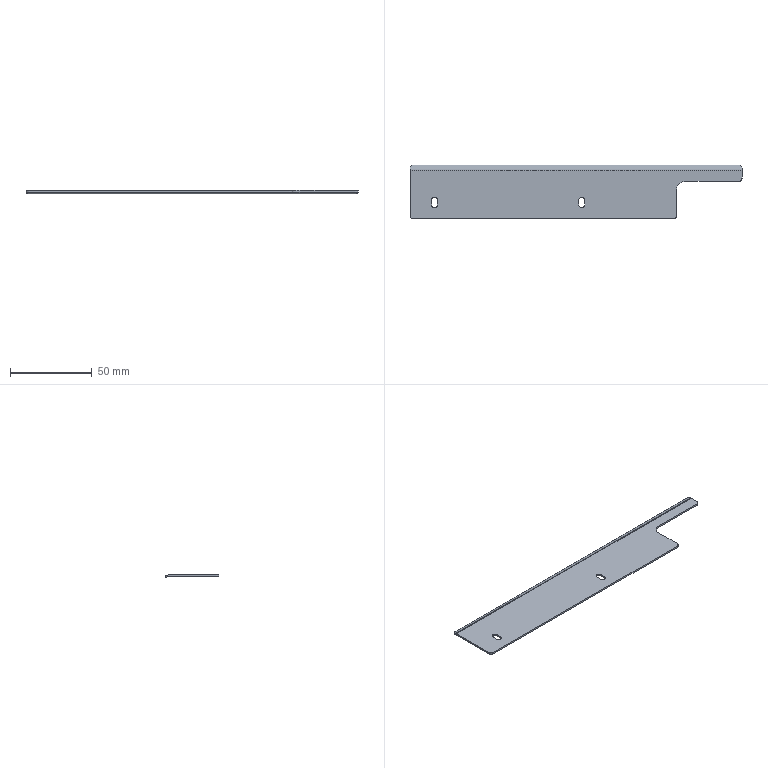Part | STEP file | 01-16 side baffle (Default) | 1 solid | 30 faces | box 203 x 32.995 x 1.966 mm | volume 5739 mm3 | plane 18 | cylinder 12 | commonest cylinder face diameters 4 x5 3.5 x4 1.473 x1 3.473 x1 10 x1
STEP:
#1=CARTESIAN_POINT('',(101.5,10.,0.));
#2=VERTEX_POINT('',#1);
#3=CARTESIAN_POINT('',(101.5,14.87,0.));
#4=VERTEX_POINT('',#3);
#5=CARTESIAN_POINT('',(101.5,15.,0.));
#6=DIRECTION('',(0.,1.,0.));
#7=VECTOR('',#6,1000.);
#8=LINE('',#5,#7);
#9=EDGE_CURVE('',#2,#4,#8,.T.);
#10=ORIENTED_EDGE('',*,*,#9,.F.);
#11=CARTESIAN_POINT('',(101.5,10.,-1.));
#12=VERTEX_POINT('',#11);
#13=CARTESIAN_POINT('',(101.5,10.,-1.));
#14=DIRECTION('',(0.,0.,-1.));
#15=VECTOR('',#14,1000.);
#16=LINE('',#13,#15);
#17=EDGE_CURVE('',#2,#12,#16,.T.);
#18=ORIENTED_EDGE('',*,*,#17,.T.);
#19=CARTESIAN_POINT('',(101.5,14.87,-1.));
#20=VERTEX_POINT('',#19);
#21=CARTESIAN_POINT('',(101.5,15.,-1.));
#22=DIRECTION('',(0.,1.,0.));
#23=VECTOR('',#22,1000.);
#24=LINE('',#21,#23);
#25=EDGE_CURVE('',#12,#20,#24,.T.);
#26=ORIENTED_EDGE('',*,*,#25,.T.);
#27=CARTESIAN_POINT('',(101.5,14.87,-1.));
#28=DIRECTION('',(0.,0.,1.));
#29=VECTOR('',#28,1000.);
#30=LINE('',#27,#29);
#31=EDGE_CURVE('',#20,#4,#30,.T.);
#32=ORIENTED_EDGE('',*,*,#31,.T.);
#33=EDGE_LOOP('',(#10,#18,#26,#32));
#34=FACE_OUTER_BOUND('',#33,.T.);
#35=CARTESIAN_POINT('',(101.5,15.,-1.));
#36=DIRECTION('',(1.,0.,0.));
#37=DIRECTION('',(0.,1.,0.));
#38=AXIS2_PLACEMENT_3D('',#35,#36,#37);
#39=PLANE('',#38);
#40=ADVANCED_FACE('',(#34),#39,.T.);
#41=CARTESIAN_POINT('',(5.25,-3.5,-1.));
#42=VERTEX_POINT('',#41);
#43=CARTESIAN_POINT('',(5.25,-6.5,-1.));
#44=VERTEX_POINT('',#43);
#45=CARTESIAN_POINT('',(5.25,-3.5,-1.));
#46=DIRECTION('',(0.,-1.,0.));
#47=VECTOR('',#46,1000.);
#48=LINE('',#45,#47);
#49=EDGE_CURVE('',#42,#44,#48,.T.);
#50=ORIENTED_EDGE('',*,*,#49,.F.);
#51=CARTESIAN_POINT('',(1.75,-3.5,-1.));
#52=VERTEX_POINT('',#51);
#53=CARTESIAN_POINT('',(3.5,-3.5,-1.));
#54=DIRECTION('',(0.,0.,-1.));
#55=DIRECTION('',(-1.,0.,0.));
#56=AXIS2_PLACEMENT_3D('',#53,#54,#55);
#57=CIRCLE('',#56,1.75);
#58=EDGE_CURVE('',#52,#42,#57,.T.);
#59=ORIENTED_EDGE('',*,*,#58,.F.);
#60=CARTESIAN_POINT('',(1.75,-6.5,-1.));
#61=VERTEX_POINT('',#60);
#62=CARTESIAN_POINT('',(1.75,-3.5,-1.));
#63=DIRECTION('',(0.,1.,0.));
#64=VECTOR('',#63,1000.);
#65=LINE('',#62,#64);
#66=EDGE_CURVE('',#61,#52,#65,.T.);
#67=ORIENTED_EDGE('',*,*,#66,.F.);
#68=CARTESIAN_POINT('',(3.5,-6.5,-1.));
#69=DIRECTION('',(0.,0.,-1.));
#70=DIRECTION('',(-1.,0.,0.));
#71=AXIS2_PLACEMENT_3D('',#68,#69,#70);
#72=CIRCLE('',#71,1.75);
#73=EDGE_CURVE('',#44,#61,#72,.T.);
#74=ORIENTED_EDGE('',*,*,#73,.F.);
#75=EDGE_LOOP('',(#50,#59,#67,#74));
#76=FACE_BOUND('',#75,.T.);
#77=CARTESIAN_POINT('',(-84.75,-3.5,-1.));
#78=VERTEX_POINT('',#77);
#79=CARTESIAN_POINT('',(-84.75,-6.5,-1.));
#80=VERTEX_POINT('',#79);
#81=CARTESIAN_POINT('',(-84.75,-3.5,-1.));
#82=DIRECTION('',(0.,-1.,0.));
#83=VECTOR('',#82,1000.);
#84=LINE('',#81,#83);
#85=EDGE_CURVE('',#78,#80,#84,.T.);
#86=ORIENTED_EDGE('',*,*,#85,.F.);
#87=CARTESIAN_POINT('',(-88.25,-3.5,-1.));
#88=VERTEX_POINT('',#87);
#89=CARTESIAN_POINT('',(-86.5,-3.5,-1.));
#90=DIRECTION('',(0.,0.,-1.));
#91=DIRECTION('',(-1.,0.,0.));
#92=AXIS2_PLACEMENT_3D('',#89,#90,#91);
#93=CIRCLE('',#92,1.75);
#94=EDGE_CURVE('',#88,#78,#93,.T.);
#95=ORIENTED_EDGE('',*,*,#94,.F.);
#96=CARTESIAN_POINT('',(-88.25,-6.5,-1.));
#97=VERTEX_POINT('',#96);
#98=CARTESIAN_POINT('',(-88.25,-3.5,-1.));
#99=DIRECTION('',(0.,1.,0.));
#100=VECTOR('',#99,1000.);
#101=LINE('',#98,#100);
#102=EDGE_CURVE('',#97,#88,#101,.T.);
#103=ORIENTED_EDGE('',*,*,#102,.F.);
#104=CARTESIAN_POINT('',(-86.5,-6.5,-1.));
#105=DIRECTION('',(0.,0.,-1.));
#106=DIRECTION('',(-1.,0.,0.));
#107=AXIS2_PLACEMENT_3D('',#104,#105,#106);
#108=CIRCLE('',#107,1.75);
#109=EDGE_CURVE('',#80,#97,#108,.T.);
#110=ORIENTED_EDGE('',*,*,#109,.F.);
#111=EDGE_LOOP('',(#86,#95,#103,#110));
#112=FACE_BOUND('',#111,.T.);
#113=ORIENTED_EDGE('',*,*,#25,.F.);
#114=CARTESIAN_POINT('',(99.5,8.,-1.));
#115=VERTEX_POINT('',#114);
#116=CARTESIAN_POINT('',(99.5,10.,-1.));
#117=DIRECTION('',(0.,0.,-1.));
#118=DIRECTION('',(1.,0.,0.));
#119=AXIS2_PLACEMENT_3D('',#116,#117,#118);
#120=CIRCLE('',#119,2.);
#121=EDGE_CURVE('',#12,#115,#120,.T.);
#122=ORIENTED_EDGE('',*,*,#121,.T.);
#123=CARTESIAN_POINT('',(66.5,8.,-1.));
#124=VERTEX_POINT('',#123);
#125=CARTESIAN_POINT('',(101.5,8.,-1.));
#126=DIRECTION('',(1.,0.,0.));
#127=VECTOR('',#126,1000.);
#128=LINE('',#125,#127);
#129=EDGE_CURVE('',#124,#115,#128,.T.);
#130=ORIENTED_EDGE('',*,*,#129,.F.);
#131=CARTESIAN_POINT('',(61.5,3.,-1.));
#132=VERTEX_POINT('',#131);
#133=CARTESIAN_POINT('',(66.5,3.,-1.));
#134=DIRECTION('',(0.,0.,-1.));
#135=DIRECTION('',(1.,0.,0.));
#136=AXIS2_PLACEMENT_3D('',#133,#134,#135);
#137=CIRCLE('',#136,5.);
#138=EDGE_CURVE('',#132,#124,#137,.T.);
#139=ORIENTED_EDGE('',*,*,#138,.F.);
#140=CARTESIAN_POINT('',(61.5,-13.,-1.));
#141=VERTEX_POINT('',#140);
#142=CARTESIAN_POINT('',(61.5,3.,-1.));
#143=DIRECTION('',(0.,1.,0.));
#144=VECTOR('',#143,1000.);
#145=LINE('',#142,#144);
#146=EDGE_CURVE('',#141,#132,#145,.T.);
#147=ORIENTED_EDGE('',*,*,#146,.F.);
#148=CARTESIAN_POINT('',(59.5,-15.,-1.));
#149=VERTEX_POINT('',#148);
#150=CARTESIAN_POINT('',(59.5,-13.,-1.));
#151=DIRECTION('',(0.,0.,-1.));
#152=DIRECTION('',(1.,0.,0.));
#153=AXIS2_PLACEMENT_3D('',#150,#151,#152);
#154=CIRCLE('',#153,2.);
#155=EDGE_CURVE('',#141,#149,#154,.T.);
#156=ORIENTED_EDGE('',*,*,#155,.T.);
#157=CARTESIAN_POINT('',(-99.5,-15.,-1.));
#158=VERTEX_POINT('',#157);
#159=CARTESIAN_POINT('',(-101.5,-15.,-1.));
#160=DIRECTION('',(1.,0.,0.));
#161=VECTOR('',#160,1000.);
#162=LINE('',#159,#161);
#163=EDGE_CURVE('',#158,#149,#162,.T.);
#164=ORIENTED_EDGE('',*,*,#163,.F.);
#165=CARTESIAN_POINT('',(-101.5,-13.,-1.));
#166=VERTEX_POINT('',#165);
#167=CARTESIAN_POINT('',(-99.5,-13.,-1.));
#168=DIRECTION('',(0.,0.,-1.));
#169=DIRECTION('',(1.,0.,0.));
#170=AXIS2_PLACEMENT_3D('',#167,#168,#169);
#171=CIRCLE('',#170,2.);
#172=EDGE_CURVE('',#158,#166,#171,.T.);
#173=ORIENTED_EDGE('',*,*,#172,.T.);
#174=CARTESIAN_POINT('',(-101.5,14.87,-1.));
#175=VERTEX_POINT('',#174);
#176=CARTESIAN_POINT('',(-101.5,15.,-1.));
#177=DIRECTION('',(0.,-1.,0.));
#178=VECTOR('',#177,1000.);
#179=LINE('',#176,#178);
#180=EDGE_CURVE('',#175,#166,#179,.T.);
#181=ORIENTED_EDGE('',*,*,#180,.F.);
#182=CARTESIAN_POINT('',(101.5,14.87,-1.));
#183=DIRECTION('',(-1.,0.,0.));
#184=VECTOR('',#183,1000.);
#185=LINE('',#182,#184);
#186=EDGE_CURVE('',#20,#175,#185,.T.);
#187=ORIENTED_EDGE('',*,*,#186,.F.);
#188=EDGE_LOOP('',(#113,#122,#130,#139,#147,#156,#164,#173,#181,#187));
#189=FACE_OUTER_BOUND('',#188,.T.);
#190=CARTESIAN_POINT('',(101.5,-15.,-1.));
#191=DIRECTION('',(0.,0.,1.));
#192=DIRECTION('',(1.,0.,0.));
#193=AXIS2_PLACEMENT_3D('',#190,#191,#192);
#194=PLANE('',#193);
#195=ADVANCED_FACE('',(#76,#112,#189),#194,.F.);
#196=CARTESIAN_POINT('',(5.25,-3.5,0.));
#197=VERTEX_POINT('',#196);
#198=CARTESIAN_POINT('',(1.75,-3.5,0.));
#199=VERTEX_POINT('',#198);
#200=CARTESIAN_POINT('',(3.5,-3.5,0.));
#201=DIRECTION('',(0.,0.,1.));
#202=DIRECTION('',(1.,0.,0.));
#203=AXIS2_PLACEMENT_3D('',#200,#201,#202);
#204=CIRCLE('',#203,1.75);
#205=EDGE_CURVE('',#197,#199,#204,.T.);
#206=ORIENTED_EDGE('',*,*,#205,.F.);
#207=CARTESIAN_POINT('',(5.25,-6.5,0.));
#208=VERTEX_POINT('',#207);
#209=CARTESIAN_POINT('',(5.25,-15.,0.));
#210=DIRECTION('',(0.,1.,0.));
#211=VECTOR('',#210,1000.);
#212=LINE('',#209,#211);
#213=EDGE_CURVE('',#208,#197,#212,.T.);
#214=ORIENTED_EDGE('',*,*,#213,.F.);
#215=CARTESIAN_POINT('',(1.75,-6.5,0.));
#216=VERTEX_POINT('',#215);
#217=CARTESIAN_POINT('',(3.5,-6.5,0.));
#218=DIRECTION('',(0.,0.,1.));
#219=DIRECTION('',(1.,0.,0.));
#220=AXIS2_PLACEMENT_3D('',#217,#218,#219);
#221=CIRCLE('',#220,1.75);
#222=EDGE_CURVE('',#216,#208,#221,.T.);
#223=ORIENTED_EDGE('',*,*,#222,.F.);
#224=CARTESIAN_POINT('',(1.75,-15.,0.));
#225=DIRECTION('',(0.,-1.,0.));
#226=VECTOR('',#225,1000.);
#227=LINE('',#224,#226);
#228=EDGE_CURVE('',#199,#216,#227,.T.);
#229=ORIENTED_EDGE('',*,*,#228,.F.);
#230=EDGE_LOOP('',(#206,#214,#223,#229));
#231=FACE_BOUND('',#230,.T.);
#232=CARTESIAN_POINT('',(-84.75,-3.5,0.));
#233=VERTEX_POINT('',#232);
#234=CARTESIAN_POINT('',(-88.25,-3.5,0.));
#235=VERTEX_POINT('',#234);
#236=CARTESIAN_POINT('',(-86.5,-3.5,0.));
#237=DIRECTION('',(0.,0.,1.));
#238=DIRECTION('',(1.,0.,0.));
#239=AXIS2_PLACEMENT_3D('',#236,#237,#238);
#240=CIRCLE('',#239,1.75);
#241=EDGE_CURVE('',#233,#235,#240,.T.);
#242=ORIENTED_EDGE('',*,*,#241,.F.);
#243=CARTESIAN_POINT('',(-84.75,-6.5,0.));
#244=VERTEX_POINT('',#243);
#245=CARTESIAN_POINT('',(-84.75,-15.,0.));
#246=DIRECTION('',(0.,1.,0.));
#247=VECTOR('',#246,1000.);
#248=LINE('',#245,#247);
#249=EDGE_CURVE('',#244,#233,#248,.T.);
#250=ORIENTED_EDGE('',*,*,#249,.F.);
#251=CARTESIAN_POINT('',(-88.25,-6.5,0.));
#252=VERTEX_POINT('',#251);
#253=CARTESIAN_POINT('',(-86.5,-6.5,0.));
#254=DIRECTION('',(0.,0.,1.));
#255=DIRECTION('',(1.,0.,0.));
#256=AXIS2_PLACEMENT_3D('',#253,#254,#255);
#257=CIRCLE('',#256,1.75);
#258=EDGE_CURVE('',#252,#244,#257,.T.);
#259=ORIENTED_EDGE('',*,*,#258,.F.);
#260=CARTESIAN_POINT('',(-88.25,-15.,0.));
#261=DIRECTION('',(0.,-1.,0.));
#262=VECTOR('',#261,1000.);
#263=LINE('',#260,#262);
#264=EDGE_CURVE('',#235,#252,#263,.T.);
#265=ORIENTED_EDGE('',*,*,#264,.F.);
#266=EDGE_LOOP('',(#242,#250,#259,#265));
#267=FACE_BOUND('',#266,.T.);
#268=CARTESIAN_POINT('',(99.5,8.,0.));
#269=VERTEX_POINT('',#268);
#270=CARTESIAN_POINT('',(66.5,8.,0.));
#271=VERTEX_POINT('',#270);
#272=CARTESIAN_POINT('',(101.5,8.,0.));
#273=DIRECTION('',(-1.,0.,0.));
#274=VECTOR('',#273,1000.);
#275=LINE('',#272,#274);
#276=EDGE_CURVE('',#269,#271,#275,.T.);
#277=ORIENTED_EDGE('',*,*,#276,.F.);
#278=CARTESIAN_POINT('',(99.5,10.,0.));
#279=DIRECTION('',(0.,0.,1.));
#280=DIRECTION('',(1.,0.,0.));
#281=AXIS2_PLACEMENT_3D('',#278,#279,#280);
#282=CIRCLE('',#281,2.);
#283=EDGE_CURVE('',#269,#2,#282,.T.);
#284=ORIENTED_EDGE('',*,*,#283,.T.);
#285=ORIENTED_EDGE('',*,*,#9,.T.);
#286=CARTESIAN_POINT('',(-101.5,14.87,0.));
#287=VERTEX_POINT('',#286);
#288=CARTESIAN_POINT('',(101.5,14.87,0.));
#289=DIRECTION('',(-1.,0.,0.));
#290=VECTOR('',#289,1000.);
#291=LINE('',#288,#290);
#292=EDGE_CURVE('',#4,#287,#291,.T.);
#293=ORIENTED_EDGE('',*,*,#292,.T.);
#294=CARTESIAN_POINT('',(-101.5,-13.,0.));
#295=VERTEX_POINT('',#294);
#296=CARTESIAN_POINT('',(-101.5,15.,0.));
#297=DIRECTION('',(0.,-1.,0.));
#298=VECTOR('',#297,1000.);
#299=LINE('',#296,#298);
#300=EDGE_CURVE('',#287,#295,#299,.T.);
#301=ORIENTED_EDGE('',*,*,#300,.T.);
#302=CARTESIAN_POINT('',(-99.5,-15.,0.));
#303=VERTEX_POINT('',#302);
#304=CARTESIAN_POINT('',(-99.5,-13.,0.));
#305=DIRECTION('',(0.,0.,1.));
#306=DIRECTION('',(1.,0.,0.));
#307=AXIS2_PLACEMENT_3D('',#304,#305,#306);
#308=CIRCLE('',#307,2.);
#309=EDGE_CURVE('',#295,#303,#308,.T.);
#310=ORIENTED_EDGE('',*,*,#309,.T.);
#311=CARTESIAN_POINT('',(59.5,-15.,0.));
#312=VERTEX_POINT('',#311);
#313=CARTESIAN_POINT('',(-101.5,-15.,0.));
#314=DIRECTION('',(1.,0.,0.));
#315=VECTOR('',#314,1000.);
#316=LINE('',#313,#315);
#317=EDGE_CURVE('',#303,#312,#316,.T.);
#318=ORIENTED_EDGE('',*,*,#317,.T.);
#319=CARTESIAN_POINT('',(61.5,-13.,0.));
#320=VERTEX_POINT('',#319);
#321=CARTESIAN_POINT('',(59.5,-13.,0.));
#322=DIRECTION('',(0.,0.,1.));
#323=DIRECTION('',(1.,0.,0.));
#324=AXIS2_PLACEMENT_3D('',#321,#322,#323);
#325=CIRCLE('',#324,2.);
#326=EDGE_CURVE('',#312,#320,#325,.T.);
#327=ORIENTED_EDGE('',*,*,#326,.T.);
#328=CARTESIAN_POINT('',(61.5,3.,0.));
#329=VERTEX_POINT('',#328);
#330=CARTESIAN_POINT('',(61.5,-15.,0.));
#331=DIRECTION('',(0.,-1.,0.));
#332=VECTOR('',#331,1000.);
#333=LINE('',#330,#332);
#334=EDGE_CURVE('',#329,#320,#333,.T.);
#335=ORIENTED_EDGE('',*,*,#334,.F.);
#336=CARTESIAN_POINT('',(66.5,3.,0.));
#337=DIRECTION('',(0.,0.,1.));
#338=DIRECTION('',(1.,0.,0.));
#339=AXIS2_PLACEMENT_3D('',#336,#337,#338);
#340=CIRCLE('',#339,5.);
#341=EDGE_CURVE('',#271,#329,#340,.T.);
#342=ORIENTED_EDGE('',*,*,#341,.F.);
#343=EDGE_LOOP('',(#277,#284,#285,#293,#301,#310,#318,#327,#335,#342));
#344=FACE_OUTER_BOUND('',#343,.T.);
#345=CARTESIAN_POINT('',(101.5,-15.,0.));
#346=DIRECTION('',(0.,0.,1.));
#347=DIRECTION('',(1.,0.,0.));
#348=AXIS2_PLACEMENT_3D('',#345,#346,#347);
#349=PLANE('',#348);
#350=ADVANCED_FACE('',(#231,#267,#344),#349,.T.);
#351=ORIENTED_EDGE('',*,*,#163,.T.);
#352=CARTESIAN_POINT('',(59.5,-15.,0.));
#353=DIRECTION('',(0.,0.,1.));
#354=VECTOR('',#353,1000.);
#355=LINE('',#352,#354);
#356=EDGE_CURVE('',#149,#312,#355,.T.);
#357=ORIENTED_EDGE('',*,*,#356,.T.);
#358=ORIENTED_EDGE('',*,*,#317,.F.);
#359=CARTESIAN_POINT('',(-99.5,-15.,-1.));
#360=DIRECTION('',(0.,0.,-1.));
#361=VECTOR('',#360,1000.);
#362=LINE('',#359,#361);
#363=EDGE_CURVE('',#303,#158,#362,.T.);
#364=ORIENTED_EDGE('',*,*,#363,.T.);
#365=EDGE_LOOP('',(#351,#357,#358,#364));
#366=FACE_OUTER_BOUND('',#365,.T.);
#367=CARTESIAN_POINT('',(-101.5,-15.,-1.));
#368=DIRECTION('',(0.,-1.,0.));
#369=DIRECTION('',(0.,0.,-1.));
#370=AXIS2_PLACEMENT_3D('',#367,#368,#369);
#371=PLANE('',#370);
#372=ADVANCED_FACE('',(#366),#371,.T.);
#373=ORIENTED_EDGE('',*,*,#180,.T.);
#374=CARTESIAN_POINT('',(-101.5,-13.,-1.));
#375=DIRECTION('',(0.,0.,1.));
#376=VECTOR('',#375,1000.);
#377=LINE('',#374,#376);
#378=EDGE_CURVE('',#166,#295,#377,.T.);
#379=ORIENTED_EDGE('',*,*,#378,.T.);
#380=ORIENTED_EDGE('',*,*,#300,.F.);
#381=CARTESIAN_POINT('',(-101.5,14.87,-1.));
#382=DIRECTION('',(0.,0.,1.));
#383=VECTOR('',#382,1000.);
#384=LINE('',#381,#383);
#385=EDGE_CURVE('',#175,#287,#384,.T.);
#386=ORIENTED_EDGE('',*,*,#385,.F.);
#387=EDGE_LOOP('',(#373,#379,#380,#386));
#388=FACE_OUTER_BOUND('',#387,.T.);
#389=CARTESIAN_POINT('',(-101.5,15.,-1.));
#390=DIRECTION('',(-1.,0.,0.));
#391=DIRECTION('',(0.,0.,1.));
#392=AXIS2_PLACEMENT_3D('',#389,#390,#391);
#393=PLANE('',#392);
#394=ADVANCED_FACE('',(#388),#393,.T.);
#395=CARTESIAN_POINT('',(-101.5,15.122,-1.044));
#396=VERTEX_POINT('',#395);
#397=CARTESIAN_POINT('',(-101.5,15.464,-0.1047));
#398=VERTEX_POINT('',#397);
#399=CARTESIAN_POINT('',(-101.5,15.122,-1.044));
#400=DIRECTION('',(0.,0.342,0.9397));
#401=VECTOR('',#400,1000.);
#402=LINE('',#399,#401);
#403=EDGE_CURVE('',#396,#398,#402,.T.);
#404=ORIENTED_EDGE('',*,*,#403,.F.);
#405=CARTESIAN_POINT('',(-101.5,14.87,-1.737));
#406=DIRECTION('',(-1.,0.,0.));
#407=DIRECTION('',(0.,0.,-1.));
#408=AXIS2_PLACEMENT_3D('',#405,#406,#407);
#409=CIRCLE('',#408,0.7366);
#410=EDGE_CURVE('',#175,#396,#409,.T.);
#411=ORIENTED_EDGE('',*,*,#410,.F.);
#412=ORIENTED_EDGE('',*,*,#385,.T.);
#413=CARTESIAN_POINT('',(-101.5,14.87,-1.737));
#414=DIRECTION('',(-1.,0.,0.));
#415=DIRECTION('',(0.,0.,-1.));
#416=AXIS2_PLACEMENT_3D('',#413,#414,#415);
#417=CIRCLE('',#416,1.737);
#418=EDGE_CURVE('',#287,#398,#417,.T.);
#419=ORIENTED_EDGE('',*,*,#418,.T.);
#420=EDGE_LOOP('',(#404,#411,#412,#419));
#421=FACE_OUTER_BOUND('',#420,.T.);
#422=CARTESIAN_POINT('',(-101.5,14.87,-1.737));
#423=DIRECTION('',(-1.,0.,0.));
#424=DIRECTION('',(0.,0.,1.));
#425=AXIS2_PLACEMENT_3D('',#422,#423,#424);
#426=PLANE('',#425);
#427=ADVANCED_FACE('',(#421),#426,.T.);
#428=CARTESIAN_POINT('',(101.5,15.122,-1.044));
#429=VERTEX_POINT('',#428);
#430=CARTESIAN_POINT('',(101.5,14.87,-1.737));
#431=DIRECTION('',(1.,0.,0.));
#432=DIRECTION('',(0.,0.,-1.));
#433=AXIS2_PLACEMENT_3D('',#430,#431,#432);
#434=CIRCLE('',#433,0.7366);
#435=EDGE_CURVE('',#429,#20,#434,.T.);
#436=ORIENTED_EDGE('',*,*,#435,.F.);
#437=CARTESIAN_POINT('',(101.5,15.464,-0.1047));
#438=VERTEX_POINT('',#437);
#439=CARTESIAN_POINT('',(101.5,15.122,-1.044));
#440=DIRECTION('',(0.,0.342,0.9397));
#441=VECTOR('',#440,1000.);
#442=LINE('',#439,#441);
#443=EDGE_CURVE('',#429,#438,#442,.T.);
#444=ORIENTED_EDGE('',*,*,#443,.T.);
#445=CARTESIAN_POINT('',(101.5,14.87,-1.737));
#446=DIRECTION('',(1.,0.,0.));
#447=DIRECTION('',(0.,0.,-1.));
#448=AXIS2_PLACEMENT_3D('',#445,#446,#447);
#449=CIRCLE('',#448,1.737);
#450=EDGE_CURVE('',#438,#4,#449,.T.);
#451=ORIENTED_EDGE('',*,*,#450,.T.);
#452=ORIENTED_EDGE('',*,*,#31,.F.);
#453=EDGE_LOOP('',(#436,#444,#451,#452));
#454=FACE_OUTER_BOUND('',#453,.T.);
#455=CARTESIAN_POINT('',(101.5,14.87,-1.737));
#456=DIRECTION('',(-1.,0.,0.));
#457=DIRECTION('',(0.,0.,1.));
#458=AXIS2_PLACEMENT_3D('',#455,#456,#457);
#459=PLANE('',#458);
#460=ADVANCED_FACE('',(#454),#459,.F.);
#461=ORIENTED_EDGE('',*,*,#292,.F.);
#462=ORIENTED_EDGE('',*,*,#450,.F.);
#463=CARTESIAN_POINT('',(101.5,15.464,-0.1047));
#464=DIRECTION('',(-1.,0.,0.));
#465=VECTOR('',#464,1000.);
#466=LINE('',#463,#465);
#467=EDGE_CURVE('',#438,#398,#466,.T.);
#468=ORIENTED_EDGE('',*,*,#467,.T.);
#469=ORIENTED_EDGE('',*,*,#418,.F.);
#470=EDGE_LOOP('',(#461,#462,#468,#469));
#471=FACE_OUTER_BOUND('',#470,.T.);
#472=CARTESIAN_POINT('',(101.5,14.87,-1.737));
#473=DIRECTION('',(1.,0.,0.));
#474=DIRECTION('',(0.,0.342,0.9397));
#475=AXIS2_PLACEMENT_3D('',#472,#473,#474);
#476=CYLINDRICAL_SURFACE('',#475,1.737);
#477=ADVANCED_FACE('',(#471),#476,.T.);
#478=ORIENTED_EDGE('',*,*,#186,.T.);
#479=ORIENTED_EDGE('',*,*,#410,.T.);
#480=CARTESIAN_POINT('',(-101.5,15.122,-1.044));
#481=DIRECTION('',(1.,0.,0.));
#482=VECTOR('',#481,1000.);
#483=LINE('',#480,#482);
#484=EDGE_CURVE('',#396,#429,#483,.T.);
#485=ORIENTED_EDGE('',*,*,#484,.T.);
#486=ORIENTED_EDGE('',*,*,#435,.T.);
#487=EDGE_LOOP('',(#478,#479,#485,#486));
#488=FACE_OUTER_BOUND('',#487,.T.);
#489=CARTESIAN_POINT('',(101.5,14.87,-1.737));
#490=DIRECTION('',(1.,0.,0.));
#491=DIRECTION('',(0.,0.342,0.9397));
#492=AXIS2_PLACEMENT_3D('',#489,#490,#491);
#493=CYLINDRICAL_SURFACE('',#492,0.7366);
#494=ADVANCED_FACE('',(#488),#493,.F.);
#495=CARTESIAN_POINT('',(101.5,15.774,-1.282));
#496=VERTEX_POINT('',#495);
#497=CARTESIAN_POINT('',(101.5,17.653,-1.966));
#498=DIRECTION('',(0.,0.9397,-0.342));
#499=VECTOR('',#498,1000.);
#500=LINE('',#497,#499);
#501=EDGE_CURVE('',#429,#496,#500,.T.);
#502=ORIENTED_EDGE('',*,*,#501,.T.);
#503=CARTESIAN_POINT('',(101.5,16.116,-0.342));
#504=VERTEX_POINT('',#503);
#505=CARTESIAN_POINT('',(101.5,16.116,-0.342));
#506=DIRECTION('',(0.,0.342,0.9397));
#507=VECTOR('',#506,1000.);
#508=LINE('',#505,#507);
#509=EDGE_CURVE('',#496,#504,#508,.T.);
#510=ORIENTED_EDGE('',*,*,#509,.T.);
#511=CARTESIAN_POINT('',(101.5,17.995,-1.026));
#512=DIRECTION('',(0.,0.9397,-0.342));
#513=VECTOR('',#512,1000.);
#514=LINE('',#511,#513);
#515=EDGE_CURVE('',#438,#504,#514,.T.);
#516=ORIENTED_EDGE('',*,*,#515,.F.);
#517=ORIENTED_EDGE('',*,*,#443,.F.);
#518=EDGE_LOOP('',(#502,#510,#516,#517));
#519=FACE_OUTER_BOUND('',#518,.T.);
#520=CARTESIAN_POINT('',(101.5,17.995,-1.026));
#521=DIRECTION('',(-1.,0.,0.));
#522=DIRECTION('',(0.,0.,1.));
#523=AXIS2_PLACEMENT_3D('',#520,#521,#522);
#524=PLANE('',#523);
#525=ADVANCED_FACE('',(#519),#524,.F.);
#526=CARTESIAN_POINT('',(-101.5,16.116,-0.342));
#527=VERTEX_POINT('',#526);
#528=CARTESIAN_POINT('',(-101.5,15.342,-0.06031));
#529=DIRECTION('',(0.,-0.9397,0.342));
#530=VECTOR('',#529,1000.);
#531=LINE('',#528,#530);
#532=EDGE_CURVE('',#527,#398,#531,.T.);
#533=ORIENTED_EDGE('',*,*,#532,.F.);
#534=CARTESIAN_POINT('',(-101.5,15.774,-1.282));
#535=VERTEX_POINT('',#534);
#536=CARTESIAN_POINT('',(-101.5,16.116,-0.342));
#537=DIRECTION('',(0.,-0.342,-0.9397));
#538=VECTOR('',#537,1000.);
#539=LINE('',#536,#538);
#540=EDGE_CURVE('',#527,#535,#539,.T.);
#541=ORIENTED_EDGE('',*,*,#540,.T.);
#542=CARTESIAN_POINT('',(-101.5,15.,-1.));
#543=DIRECTION('',(0.,-0.9397,0.342));
#544=VECTOR('',#543,1000.);
#545=LINE('',#542,#544);
#546=EDGE_CURVE('',#535,#396,#545,.T.);
#547=ORIENTED_EDGE('',*,*,#546,.T.);
#548=ORIENTED_EDGE('',*,*,#403,.T.);
#549=EDGE_LOOP('',(#533,#541,#547,#548));
#550=FACE_OUTER_BOUND('',#549,.T.);
#551=CARTESIAN_POINT('',(-101.5,15.342,-0.06031));
#552=DIRECTION('',(1.,0.,0.));
#553=DIRECTION('',(0.,0.,-1.));
#554=AXIS2_PLACEMENT_3D('',#551,#552,#553);
#555=PLANE('',#554);
#556=ADVANCED_FACE('',(#550),#555,.F.);
#557=ORIENTED_EDGE('',*,*,#515,.T.);
#558=CARTESIAN_POINT('',(99.5,17.995,-1.026));
#559=VERTEX_POINT('',#558);
#560=CARTESIAN_POINT('',(99.5,16.116,-0.342));
#561=DIRECTION('',(0.,0.342,0.9397));
#562=DIRECTION('',(0.,0.9397,-0.342));
#563=AXIS2_PLACEMENT_3D('',#560,#561,#562);
#564=CIRCLE('',#563,2.);
#565=EDGE_CURVE('',#504,#559,#564,.T.);
#566=ORIENTED_EDGE('',*,*,#565,.T.);
#567=CARTESIAN_POINT('',(-99.5,17.995,-1.026));
#568=VERTEX_POINT('',#567);
#569=CARTESIAN_POINT('',(-101.5,17.995,-1.026));
#570=DIRECTION('',(-1.,0.,0.));
#571=VECTOR('',#570,1000.);
#572=LINE('',#569,#571);
#573=EDGE_CURVE('',#559,#568,#572,.T.);
#574=ORIENTED_EDGE('',*,*,#573,.T.);
#575=CARTESIAN_POINT('',(-99.5,16.116,-0.342));
#576=DIRECTION('',(0.,0.342,0.9397));
#577=DIRECTION('',(0.,0.9397,-0.342));
#578=AXIS2_PLACEMENT_3D('',#575,#576,#577);
#579=CIRCLE('',#578,2.);
#580=EDGE_CURVE('',#568,#527,#579,.T.);
#581=ORIENTED_EDGE('',*,*,#580,.T.);
#582=ORIENTED_EDGE('',*,*,#532,.T.);
#583=ORIENTED_EDGE('',*,*,#467,.F.);
#584=EDGE_LOOP('',(#557,#566,#574,#581,#582,#583));
#585=FACE_OUTER_BOUND('',#584,.T.);
#586=CARTESIAN_POINT('',(101.5,15.342,-0.06031));
#587=DIRECTION('',(0.,-0.342,-0.9397));
#588=DIRECTION('',(0.,0.9397,-0.342));
#589=AXIS2_PLACEMENT_3D('',#586,#587,#588);
#590=PLANE('',#589);
#591=ADVANCED_FACE('',(#585),#590,.F.);
#592=CARTESIAN_POINT('',(99.5,17.653,-1.966));
#593=VERTEX_POINT('',#592);
#594=CARTESIAN_POINT('',(-99.5,17.653,-1.966));
#595=VERTEX_POINT('',#594);
#596=CARTESIAN_POINT('',(-101.5,17.653,-1.966));
#597=DIRECTION('',(-1.,0.,0.));
#598=VECTOR('',#597,1000.);
#599=LINE('',#596,#598);
#600=EDGE_CURVE('',#593,#595,#599,.T.);
#601=ORIENTED_EDGE('',*,*,#600,.F.);
#602=CARTESIAN_POINT('',(99.5,15.774,-1.282));
#603=DIRECTION('',(0.,-0.342,-0.9397));
#604=DIRECTION('',(0.,0.9397,-0.342));
#605=AXIS2_PLACEMENT_3D('',#602,#603,#604);
#606=CIRCLE('',#605,2.);
#607=EDGE_CURVE('',#593,#496,#606,.T.);
#608=ORIENTED_EDGE('',*,*,#607,.T.);
#609=ORIENTED_EDGE('',*,*,#501,.F.);
#610=ORIENTED_EDGE('',*,*,#484,.F.);
#611=ORIENTED_EDGE('',*,*,#546,.F.);
#612=CARTESIAN_POINT('',(-99.5,15.774,-1.282));
#613=DIRECTION('',(0.,-0.342,-0.9397));
#614=DIRECTION('',(0.,0.9397,-0.342));
#615=AXIS2_PLACEMENT_3D('',#612,#613,#614);
#616=CIRCLE('',#615,2.);
#617=EDGE_CURVE('',#535,#595,#616,.T.);
#618=ORIENTED_EDGE('',*,*,#617,.T.);
#619=EDGE_LOOP('',(#601,#608,#609,#610,#611,#618));
#620=FACE_OUTER_BOUND('',#619,.T.);
#621=CARTESIAN_POINT('',(101.5,15.,-1.));
#622=DIRECTION('',(0.,-0.342,-0.9397));
#623=DIRECTION('',(0.,0.9397,-0.342));
#624=AXIS2_PLACEMENT_3D('',#621,#622,#623);
#625=PLANE('',#624);
#626=ADVANCED_FACE('',(#620),#625,.T.);
#627=ORIENTED_EDGE('',*,*,#573,.F.);
#628=CARTESIAN_POINT('',(99.5,17.995,-1.026));
#629=DIRECTION('',(0.,-0.342,-0.9397));
#630=VECTOR('',#629,1000.);
#631=LINE('',#628,#630);
#632=EDGE_CURVE('',#559,#593,#631,.T.);
#633=ORIENTED_EDGE('',*,*,#632,.T.);
#634=ORIENTED_EDGE('',*,*,#600,.T.);
#635=CARTESIAN_POINT('',(-99.5,17.995,-1.026));
#636=DIRECTION('',(0.,0.342,0.9397));
#637=VECTOR('',#636,1000.);
#638=LINE('',#635,#637);
#639=EDGE_CURVE('',#595,#568,#638,.T.);
#640=ORIENTED_EDGE('',*,*,#639,.T.);
#641=EDGE_LOOP('',(#627,#633,#634,#640));
#642=FACE_OUTER_BOUND('',#641,.T.);
#643=CARTESIAN_POINT('',(-101.5,17.995,-1.026));
#644=DIRECTION('',(0.,-0.9397,0.342));
#645=DIRECTION('',(0.,-0.342,-0.9397));
#646=AXIS2_PLACEMENT_3D('',#643,#644,#645);
#647=PLANE('',#646);
#648=ADVANCED_FACE('',(#642),#647,.F.);
#649=ORIENTED_EDGE('',*,*,#172,.F.);
#650=ORIENTED_EDGE('',*,*,#363,.F.);
#651=ORIENTED_EDGE('',*,*,#309,.F.);
#652=ORIENTED_EDGE('',*,*,#378,.F.);
#653=EDGE_LOOP('',(#649,#650,#651,#652));
#654=FACE_OUTER_BOUND('',#653,.T.);
#655=CARTESIAN_POINT('',(-99.5,-13.,-1.));
#656=DIRECTION('',(0.,0.,1.));
#657=DIRECTION('',(1.,0.,0.));
#658=AXIS2_PLACEMENT_3D('',#655,#656,#657);
#659=CYLINDRICAL_SURFACE('',#658,2.);
#660=ADVANCED_FACE('',(#654),#659,.T.);
#661=ORIENTED_EDGE('',*,*,#565,.F.);
#662=ORIENTED_EDGE('',*,*,#509,.F.);
#663=ORIENTED_EDGE('',*,*,#607,.F.);
#664=ORIENTED_EDGE('',*,*,#632,.F.);
#665=EDGE_LOOP('',(#661,#662,#663,#664));
#666=FACE_OUTER_BOUND('',#665,.T.);
#667=CARTESIAN_POINT('',(99.5,16.116,-0.342));
#668=DIRECTION('',(0.,-0.342,-0.9397));
#669=DIRECTION('',(0.,0.9397,-0.342));
#670=AXIS2_PLACEMENT_3D('',#667,#668,#669);
#671=CYLINDRICAL_SURFACE('',#670,2.);
#672=ADVANCED_FACE('',(#666),#671,.T.);
#673=ORIENTED_EDGE('',*,*,#580,.F.);
#674=ORIENTED_EDGE('',*,*,#639,.F.);
#675=ORIENTED_EDGE('',*,*,#617,.F.);
#676=ORIENTED_EDGE('',*,*,#540,.F.);
#677=EDGE_LOOP('',(#673,#674,#675,#676));
#678=FACE_OUTER_BOUND('',#677,.T.);
#679=CARTESIAN_POINT('',(-99.5,16.116,-0.342));
#680=DIRECTION('',(0.,-0.342,-0.9397));
#681=DIRECTION('',(0.,0.9397,-0.342));
#682=AXIS2_PLACEMENT_3D('',#679,#680,#681);
#683=CYLINDRICAL_SURFACE('',#682,2.);
#684=ADVANCED_FACE('',(#678),#683,.T.);
#685=ORIENTED_EDGE('',*,*,#129,.T.);
#686=CARTESIAN_POINT('',(99.5,8.,0.));
#687=DIRECTION('',(0.,0.,1.));
#688=VECTOR('',#687,1000.);
#689=LINE('',#686,#688);
#690=EDGE_CURVE('',#115,#269,#689,.T.);
#691=ORIENTED_EDGE('',*,*,#690,.T.);
#692=ORIENTED_EDGE('',*,*,#276,.T.);
#693=CARTESIAN_POINT('',(66.5,8.,9.));
#694=DIRECTION('',(0.,0.,-1.));
#695=VECTOR('',#694,1000.);
#696=LINE('',#693,#695);
#697=EDGE_CURVE('',#271,#124,#696,.T.);
#698=ORIENTED_EDGE('',*,*,#697,.T.);
#699=EDGE_LOOP('',(#685,#691,#692,#698));
#700=FACE_OUTER_BOUND('',#699,.T.);
#701=CARTESIAN_POINT('',(101.5,8.,9.));
#702=DIRECTION('',(0.,1.,0.));
#703=DIRECTION('',(0.,0.,1.));
#704=AXIS2_PLACEMENT_3D('',#701,#702,#703);
#705=PLANE('',#704);
#706=ADVANCED_FACE('',(#700),#705,.F.);
#707=ORIENTED_EDGE('',*,*,#341,.T.);
#708=CARTESIAN_POINT('',(61.5,3.,9.));
#709=DIRECTION('',(0.,0.,-1.));
#710=VECTOR('',#709,1000.);
#711=LINE('',#708,#710);
#712=EDGE_CURVE('',#329,#132,#711,.T.);
#713=ORIENTED_EDGE('',*,*,#712,.T.);
#714=ORIENTED_EDGE('',*,*,#138,.T.);
#715=ORIENTED_EDGE('',*,*,#697,.F.);
#716=EDGE_LOOP('',(#707,#713,#714,#715));
#717=FACE_OUTER_BOUND('',#716,.T.);
#718=CARTESIAN_POINT('',(66.5,3.,9.));
#719=DIRECTION('',(0.,0.,-1.));
#720=DIRECTION('',(-1.,0.,0.));
#721=AXIS2_PLACEMENT_3D('',#718,#719,#720);
#722=CYLINDRICAL_SURFACE('',#721,5.);
#723=ADVANCED_FACE('',(#717),#722,.F.);
#724=ORIENTED_EDGE('',*,*,#334,.T.);
#725=CARTESIAN_POINT('',(61.5,-13.,-1.));
#726=DIRECTION('',(0.,0.,-1.));
#727=VECTOR('',#726,1000.);
#728=LINE('',#725,#727);
#729=EDGE_CURVE('',#320,#141,#728,.T.);
#730=ORIENTED_EDGE('',*,*,#729,.T.);
#731=ORIENTED_EDGE('',*,*,#146,.T.);
#732=ORIENTED_EDGE('',*,*,#712,.F.);
#733=EDGE_LOOP('',(#724,#730,#731,#732));
#734=FACE_OUTER_BOUND('',#733,.T.);
#735=CARTESIAN_POINT('',(61.5,3.,9.));
#736=DIRECTION('',(-1.,0.,0.));
#737=DIRECTION('',(0.,0.,1.));
#738=AXIS2_PLACEMENT_3D('',#735,#736,#737);
#739=PLANE('',#738);
#740=ADVANCED_FACE('',(#734),#739,.F.);
#741=ORIENTED_EDGE('',*,*,#241,.T.);
#742=CARTESIAN_POINT('',(-88.25,-3.5,9.));
#743=DIRECTION('',(0.,0.,-1.));
#744=VECTOR('',#743,1000.);
#745=LINE('',#742,#744);
#746=EDGE_CURVE('',#235,#88,#745,.T.);
#747=ORIENTED_EDGE('',*,*,#746,.T.);
#748=ORIENTED_EDGE('',*,*,#94,.T.);
#749=CARTESIAN_POINT('',(-84.75,-3.5,9.));
#750=DIRECTION('',(0.,0.,-1.));
#751=VECTOR('',#750,1000.);
#752=LINE('',#749,#751);
#753=EDGE_CURVE('',#233,#78,#752,.T.);
#754=ORIENTED_EDGE('',*,*,#753,.F.);
#755=EDGE_LOOP('',(#741,#747,#748,#754));
#756=FACE_OUTER_BOUND('',#755,.T.);
#757=CARTESIAN_POINT('',(-86.5,-3.5,9.));
#758=DIRECTION('',(0.,0.,-1.));
#759=DIRECTION('',(-1.,0.,0.));
#760=AXIS2_PLACEMENT_3D('',#757,#758,#759);
#761=CYLINDRICAL_SURFACE('',#760,1.75);
#762=ADVANCED_FACE('',(#756),#761,.F.);
#763=ORIENTED_EDGE('',*,*,#264,.T.);
#764=CARTESIAN_POINT('',(-88.25,-6.5,9.));
#765=DIRECTION('',(0.,0.,-1.));
#766=VECTOR('',#765,1000.);
#767=LINE('',#764,#766);
#768=EDGE_CURVE('',#252,#97,#767,.T.);
#769=ORIENTED_EDGE('',*,*,#768,.T.);
#770=ORIENTED_EDGE('',*,*,#102,.T.);
#771=ORIENTED_EDGE('',*,*,#746,.F.);
#772=EDGE_LOOP('',(#763,#769,#770,#771));
#773=FACE_OUTER_BOUND('',#772,.T.);
#774=CARTESIAN_POINT('',(-88.25,-3.5,9.));
#775=DIRECTION('',(-1.,0.,0.));
#776=DIRECTION('',(0.,0.,1.));
#777=AXIS2_PLACEMENT_3D('',#774,#775,#776);
#778=PLANE('',#777);
#779=ADVANCED_FACE('',(#773),#778,.F.);
#780=ORIENTED_EDGE('',*,*,#258,.T.);
#781=CARTESIAN_POINT('',(-84.75,-6.5,9.));
#782=DIRECTION('',(0.,0.,-1.));
#783=VECTOR('',#782,1000.);
#784=LINE('',#781,#783);
#785=EDGE_CURVE('',#244,#80,#784,.T.);
#786=ORIENTED_EDGE('',*,*,#785,.T.);
#787=ORIENTED_EDGE('',*,*,#109,.T.);
#788=ORIENTED_EDGE('',*,*,#768,.F.);
#789=EDGE_LOOP('',(#780,#786,#787,#788));
#790=FACE_OUTER_BOUND('',#789,.T.);
#791=CARTESIAN_POINT('',(-86.5,-6.5,9.));
#792=DIRECTION('',(0.,0.,-1.));
#793=DIRECTION('',(-1.,0.,0.));
#794=AXIS2_PLACEMENT_3D('',#791,#792,#793);
#795=CYLINDRICAL_SURFACE('',#794,1.75);
#796=ADVANCED_FACE('',(#790),#795,.F.);
#797=ORIENTED_EDGE('',*,*,#249,.T.);
#798=ORIENTED_EDGE('',*,*,#753,.T.);
#799=ORIENTED_EDGE('',*,*,#85,.T.);
#800=ORIENTED_EDGE('',*,*,#785,.F.);
#801=EDGE_LOOP('',(#797,#798,#799,#800));
#802=FACE_OUTER_BOUND('',#801,.T.);
#803=CARTESIAN_POINT('',(-84.75,-3.5,9.));
#804=DIRECTION('',(1.,0.,0.));
#805=DIRECTION('',(0.,0.,-1.));
#806=AXIS2_PLACEMENT_3D('',#803,#804,#805);
#807=PLANE('',#806);
#808=ADVANCED_FACE('',(#802),#807,.F.);
#809=ORIENTED_EDGE('',*,*,#205,.T.);
#810=CARTESIAN_POINT('',(1.75,-3.5,9.));
#811=DIRECTION('',(0.,0.,-1.));
#812=VECTOR('',#811,1000.);
#813=LINE('',#810,#812);
#814=EDGE_CURVE('',#199,#52,#813,.T.);
#815=ORIENTED_EDGE('',*,*,#814,.T.);
#816=ORIENTED_EDGE('',*,*,#58,.T.);
#817=CARTESIAN_POINT('',(5.25,-3.5,9.));
#818=DIRECTION('',(0.,0.,-1.));
#819=VECTOR('',#818,1000.);
#820=LINE('',#817,#819);
#821=EDGE_CURVE('',#197,#42,#820,.T.);
#822=ORIENTED_EDGE('',*,*,#821,.F.);
#823=EDGE_LOOP('',(#809,#815,#816,#822));
#824=FACE_OUTER_BOUND('',#823,.T.);
#825=CARTESIAN_POINT('',(3.5,-3.5,9.));
#826=DIRECTION('',(0.,0.,-1.));
#827=DIRECTION('',(-1.,0.,0.));
#828=AXIS2_PLACEMENT_3D('',#825,#826,#827);
#829=CYLINDRICAL_SURFACE('',#828,1.75);
#830=ADVANCED_FACE('',(#824),#829,.F.);
#831=ORIENTED_EDGE('',*,*,#228,.T.);
#832=CARTESIAN_POINT('',(1.75,-6.5,9.));
#833=DIRECTION('',(0.,0.,-1.));
#834=VECTOR('',#833,1000.);
#835=LINE('',#832,#834);
#836=EDGE_CURVE('',#216,#61,#835,.T.);
#837=ORIENTED_EDGE('',*,*,#836,.T.);
#838=ORIENTED_EDGE('',*,*,#66,.T.);
#839=ORIENTED_EDGE('',*,*,#814,.F.);
#840=EDGE_LOOP('',(#831,#837,#838,#839));
#841=FACE_OUTER_BOUND('',#840,.T.);
#842=CARTESIAN_POINT('',(1.75,-3.5,9.));
#843=DIRECTION('',(-1.,0.,0.));
#844=DIRECTION('',(0.,0.,1.));
#845=AXIS2_PLACEMENT_3D('',#842,#843,#844);
#846=PLANE('',#845);
#847=ADVANCED_FACE('',(#841),#846,.F.);
#848=ORIENTED_EDGE('',*,*,#222,.T.);
#849=CARTESIAN_POINT('',(5.25,-6.5,9.));
#850=DIRECTION('',(0.,0.,-1.));
#851=VECTOR('',#850,1000.);
#852=LINE('',#849,#851);
#853=EDGE_CURVE('',#208,#44,#852,.T.);
#854=ORIENTED_EDGE('',*,*,#853,.T.);
#855=ORIENTED_EDGE('',*,*,#73,.T.);
#856=ORIENTED_EDGE('',*,*,#836,.F.);
#857=EDGE_LOOP('',(#848,#854,#855,#856));
#858=FACE_OUTER_BOUND('',#857,.T.);
#859=CARTESIAN_POINT('',(3.5,-6.5,9.));
#860=DIRECTION('',(0.,0.,-1.));
#861=DIRECTION('',(-1.,0.,0.));
#862=AXIS2_PLACEMENT_3D('',#859,#860,#861);
#863=CYLINDRICAL_SURFACE('',#862,1.75);
#864=ADVANCED_FACE('',(#858),#863,.F.);
#865=ORIENTED_EDGE('',*,*,#213,.T.);
#866=ORIENTED_EDGE('',*,*,#821,.T.);
#867=ORIENTED_EDGE('',*,*,#49,.T.);
#868=ORIENTED_EDGE('',*,*,#853,.F.);
#869=EDGE_LOOP('',(#865,#866,#867,#868));
#870=FACE_OUTER_BOUND('',#869,.T.);
#871=CARTESIAN_POINT('',(5.25,-3.5,9.));
#872=DIRECTION('',(1.,0.,0.));
#873=DIRECTION('',(0.,1.,0.));
#874=AXIS2_PLACEMENT_3D('',#871,#872,#873);
#875=PLANE('',#874);
#876=ADVANCED_FACE('',(#870),#875,.F.);
#877=ORIENTED_EDGE('',*,*,#283,.F.);
#878=ORIENTED_EDGE('',*,*,#690,.F.);
#879=ORIENTED_EDGE('',*,*,#121,.F.);
#880=ORIENTED_EDGE('',*,*,#17,.F.);
#881=EDGE_LOOP('',(#877,#878,#879,#880));
#882=FACE_OUTER_BOUND('',#881,.T.);
#883=CARTESIAN_POINT('',(99.5,10.,-1.));
#884=DIRECTION('',(0.,0.,1.));
#885=DIRECTION('',(1.,0.,0.));
#886=AXIS2_PLACEMENT_3D('',#883,#884,#885);
#887=CYLINDRICAL_SURFACE('',#886,2.);
#888=ADVANCED_FACE('',(#882),#887,.T.);
#889=ORIENTED_EDGE('',*,*,#326,.F.);
#890=ORIENTED_EDGE('',*,*,#356,.F.);
#891=ORIENTED_EDGE('',*,*,#155,.F.);
#892=ORIENTED_EDGE('',*,*,#729,.F.);
#893=EDGE_LOOP('',(#889,#890,#891,#892));
#894=FACE_OUTER_BOUND('',#893,.T.);
#895=CARTESIAN_POINT('',(59.5,-13.,9.));
#896=DIRECTION('',(0.,0.,1.));
#897=DIRECTION('',(1.,0.,0.));
#898=AXIS2_PLACEMENT_3D('',#895,#896,#897);
#899=CYLINDRICAL_SURFACE('',#898,2.);
#900=ADVANCED_FACE('',(#894),#899,.T.);
#901=CLOSED_SHELL('',(#40,#195,#350,#372,#394,#427,#460,#477,#494,#525,#556,#591,#626,#648,#660,#672,#684,#706,#723,#740,#762,#779,#796,#808,#830,#847,#864,#876,#888,#900));
#902=MANIFOLD_SOLID_BREP('',#901);
#903=CARTESIAN_POINT('',(0.,0.,0.));
#904=DIRECTION('',(0.,0.,1.));
#905=DIRECTION('',(1.,0.,0.));
#906=AXIS2_PLACEMENT_3D('',#903,#904,#905);
#907=(LENGTH_UNIT()NAMED_UNIT(*)SI_UNIT(.MILLI.,.METRE.));
#908=UNCERTAINTY_MEASURE_WITH_UNIT(LENGTH_MEASURE(0.00001),#907,'','');
#909=(NAMED_UNIT(*)PLANE_ANGLE_UNIT()SI_UNIT($,.RADIAN.));
#910=(NAMED_UNIT(*)SI_UNIT($,.STERADIAN.)SOLID_ANGLE_UNIT());
#911=(GEOMETRIC_REPRESENTATION_CONTEXT(3)GLOBAL_UNCERTAINTY_ASSIGNED_CONTEXT((#908))GLOBAL_UNIT_ASSIGNED_CONTEXT((#907,#909,#910))REPRESENTATION_CONTEXT('',''));
#912=ADVANCED_BREP_SHAPE_REPRESENTATION('',(#902,#906),#911);